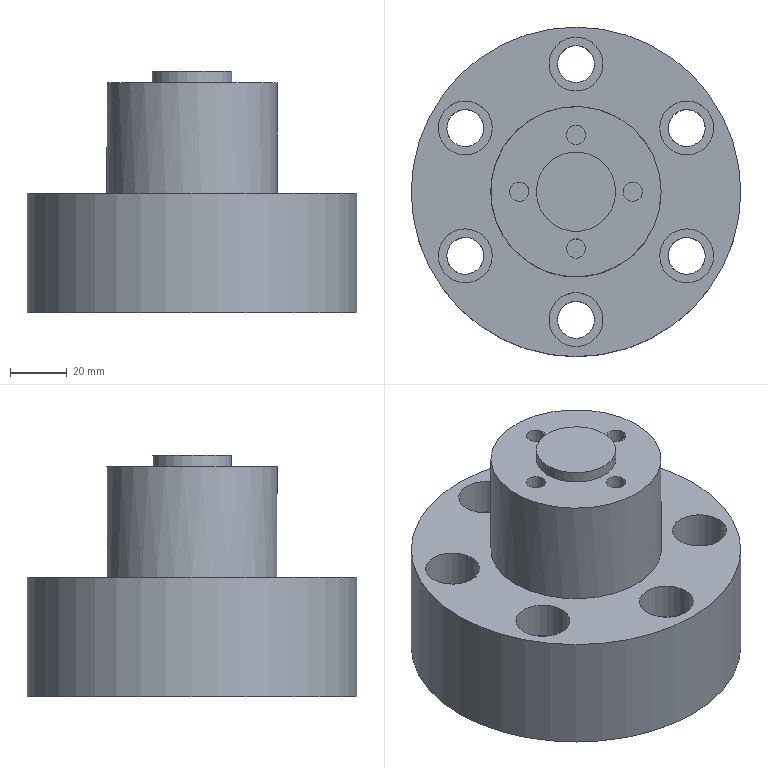CAM job | NX | 3-axis milling, drilling | part box 116 x 116 x 85 mm | stock box 116 x 116 x 85 mm
Tools:
number,name,description,diameter,corner_radius,flute_length,length,flutes
1,ZXZ,Milling Tool-5 Parameters,6.0,0.0,50.0,75.0,2
2,6.8ZT,Drilling Tool,6.8,0.0,35.0,50.0,2
3,13.0ZT,Drilling Tool,13.0,0.0,35.0,50.0,2
4,D16R0.8,Milling Tool-5 Parameters,16.0,0.8,50.0,75.0,2
Operations:
program,operation,operation_type,tool,method,geometry_group,spindle_rpm,surface_speed,feed_per_tooth,feed_cut,feed_plunge,cut_length_mm,path_length_mm,cut_time_min,machine_time_min
1,DRILLING,Operation,ZXZ,METHOD,A,3000.0,0.0,0.0,250.0,0.0,40.0,568.657,0.16,0.2129
1,DRILLING_COPY,Operation,6.8ZT,METHOD,A,2000.0,31.0,0.0375,150.0,0.0,84.172,330.672,0.5611,0.5858
1,DRILLING_COPY_COPY,Operation,13.0ZT,METHOD,A,600.0,24.0,0.125,150.0,0.0,302.434,991.367,2.016,2.085
1,HOLE_MILLING,CylinderMilling,D16R0.8,METHOD,A,2000.0,100.0,0.5,2000.0,100.0,3252.662,4425.662,1.626,1.744